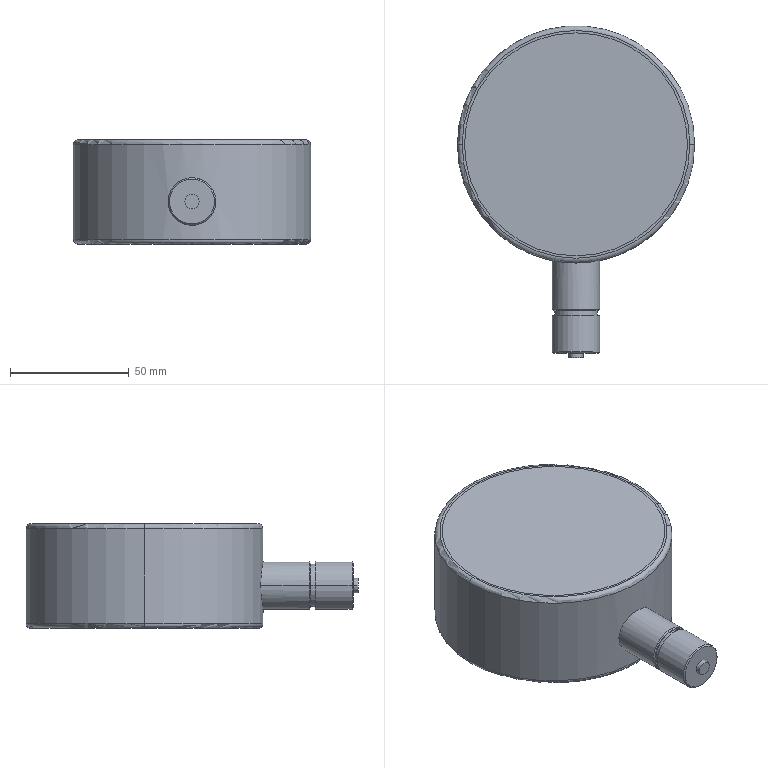Part | SolidWorks | features ICE 6, Fillet 2, Chamfer 1, Extrusion 1, MirrorPattern 1, Revolution 1 | 2 solids | 370 faces | box 100 x 140 x 44 mm | volume 86746 mm3 | plane 263 | spline 75 | cylinder 22 | torus 6 | cone 4 | commonest cylinder face diameters 6 x5 20 x4 94 x4 4.255 x3 3 x2 18 x2